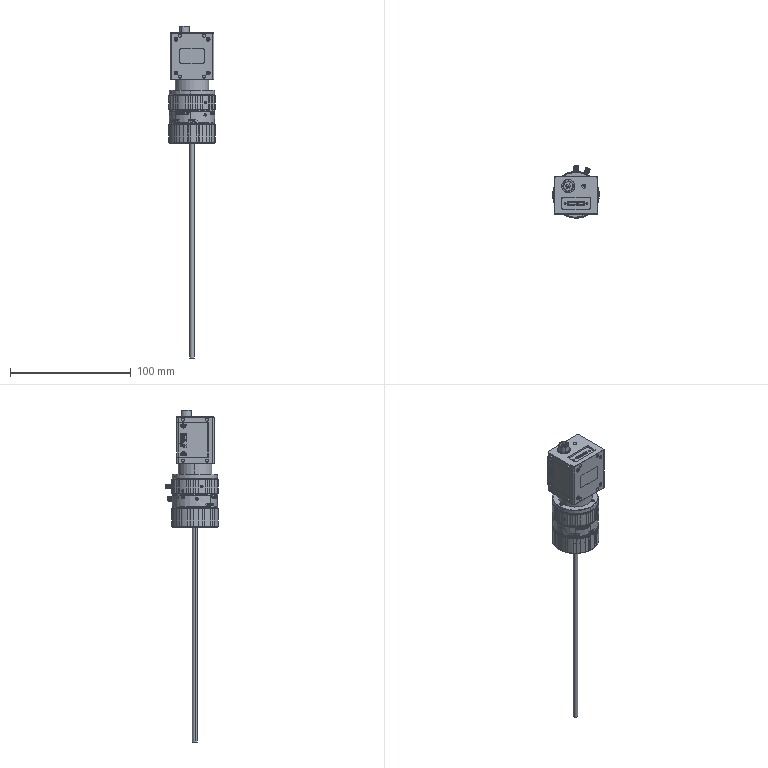Part | SolidWorks | 19 solids | 5869 faces | volume 91199 mm3 | plane 4200 | cylinder 1095 | spline 274 | cone 264 | torus 36 | commonest cylinder face diameters 1.6 x185 2 x75 4 x74 37.5 x57 1.201 x49 38.6 x43